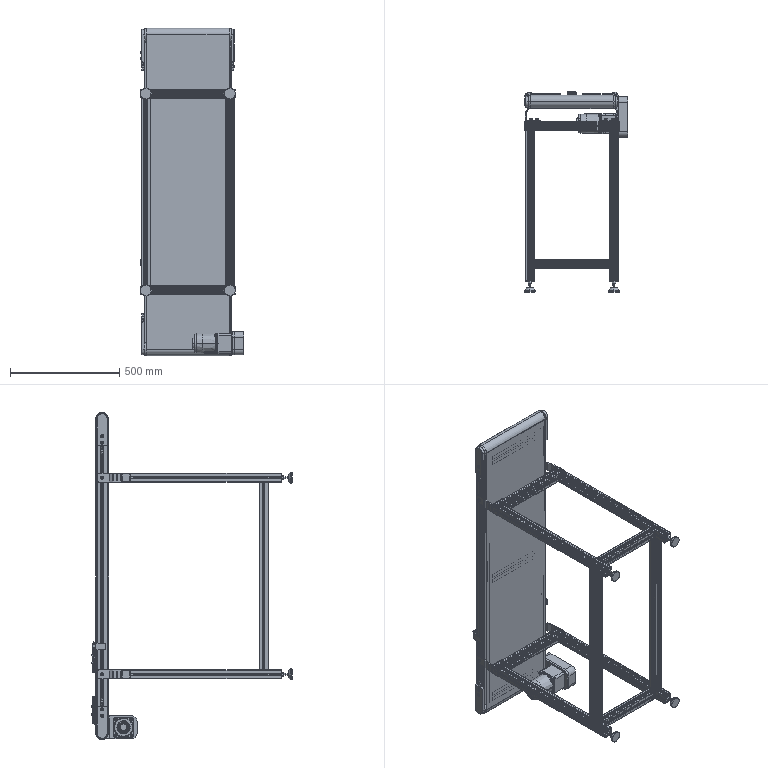Part | SolidWorks | features CoordSys 3, ReferencePattern 3, LocalLPattern 2 | 97 solids | 14026 faces | volume 14957387 mm3 | cylinder 5255 | plane 4890 | spline 2910 | torus 680 | cone 247 | sphere 44 | commonest cylinder face diameters 0.6 x2376 1 x606 2 x237 0.4 x216 0.8 x200 4 x133